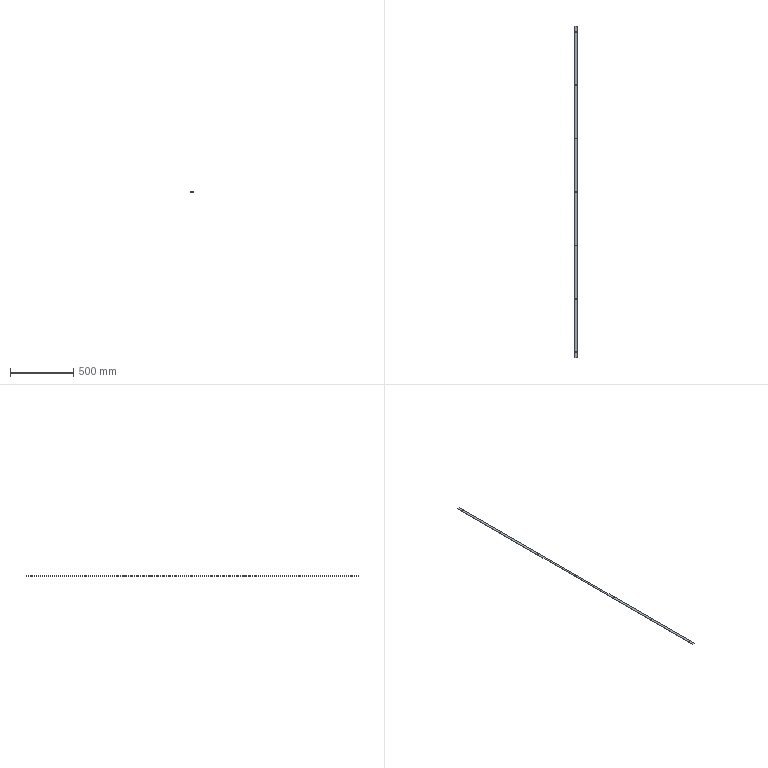Part | 1 solid | 20 faces | box 20 x 2616 x 1.5 mm | volume 78163 mm3 | cylinder 14 | plane 6 | commonest cylinder face diameters 6.2 x14
STEP:
#1=CARTESIAN_POINT('',(-3.1,-1263.,-1.5));
#2=VERTEX_POINT('',#1);
#3=CARTESIAN_POINT('',(3.1,-1263.,-1.5));
#4=VERTEX_POINT('',#3);
#5=CARTESIAN_POINT('',(0.,-1263.,-1.5));
#6=DIRECTION('',(0.,0.,1.));
#7=DIRECTION('',(1.,0.,0.));
#8=AXIS2_PLACEMENT_3D('',#5,#6,#7);
#9=CIRCLE('',#8,3.1);
#10=EDGE_CURVE('',#2,#4,#9,.T.);
#11=ORIENTED_EDGE('',*,*,#10,.F.);
#12=CARTESIAN_POINT('',(-3.1,-1263.,0.));
#13=VERTEX_POINT('',#12);
#14=CARTESIAN_POINT('',(-3.1,-1263.,-10.));
#15=DIRECTION('',(0.,0.,1.));
#16=VECTOR('',#15,1000.);
#17=LINE('',#14,#16);
#18=EDGE_CURVE('',#2,#13,#17,.T.);
#19=ORIENTED_EDGE('',*,*,#18,.T.);
#20=CARTESIAN_POINT('',(3.1,-1263.,0.));
#21=VERTEX_POINT('',#20);
#22=CARTESIAN_POINT('',(0.,-1263.,0.));
#23=DIRECTION('',(0.,0.,1.));
#24=DIRECTION('',(-1.,0.,0.));
#25=AXIS2_PLACEMENT_3D('',#22,#23,#24);
#26=CIRCLE('',#25,3.1);
#27=EDGE_CURVE('',#13,#21,#26,.T.);
#28=ORIENTED_EDGE('',*,*,#27,.T.);
#29=CARTESIAN_POINT('',(3.1,-1263.,-10.));
#30=DIRECTION('',(0.,0.,1.));
#31=VECTOR('',#30,1000.);
#32=LINE('',#29,#31);
#33=EDGE_CURVE('',#4,#21,#32,.T.);
#34=ORIENTED_EDGE('',*,*,#33,.F.);
#35=EDGE_LOOP('',(#11,#19,#28,#34));
#36=FACE_OUTER_BOUND('',#35,.T.);
#37=CARTESIAN_POINT('',(0.,-1263.,-10.));
#38=DIRECTION('',(0.,0.,1.));
#39=DIRECTION('',(1.,0.,0.));
#40=AXIS2_PLACEMENT_3D('',#37,#38,#39);
#41=CYLINDRICAL_SURFACE('',#40,3.1);
#42=ADVANCED_FACE('',(#36),#41,.F.);
#43=CARTESIAN_POINT('',(-3.1,-842.,-1.5));
#44=VERTEX_POINT('',#43);
#45=CARTESIAN_POINT('',(3.1,-842.,-1.5));
#46=VERTEX_POINT('',#45);
#47=CARTESIAN_POINT('',(0.,-842.,-1.5));
#48=DIRECTION('',(0.,0.,1.));
#49=DIRECTION('',(1.,0.,0.));
#50=AXIS2_PLACEMENT_3D('',#47,#48,#49);
#51=CIRCLE('',#50,3.1);
#52=EDGE_CURVE('',#44,#46,#51,.T.);
#53=ORIENTED_EDGE('',*,*,#52,.F.);
#54=CARTESIAN_POINT('',(-3.1,-842.,0.));
#55=VERTEX_POINT('',#54);
#56=CARTESIAN_POINT('',(-3.1,-842.,-10.));
#57=DIRECTION('',(0.,0.,1.));
#58=VECTOR('',#57,1000.);
#59=LINE('',#56,#58);
#60=EDGE_CURVE('',#44,#55,#59,.T.);
#61=ORIENTED_EDGE('',*,*,#60,.T.);
#62=CARTESIAN_POINT('',(3.1,-842.,0.));
#63=VERTEX_POINT('',#62);
#64=CARTESIAN_POINT('',(0.,-842.,0.));
#65=DIRECTION('',(0.,0.,1.));
#66=DIRECTION('',(-1.,0.,0.));
#67=AXIS2_PLACEMENT_3D('',#64,#65,#66);
#68=CIRCLE('',#67,3.1);
#69=EDGE_CURVE('',#55,#63,#68,.T.);
#70=ORIENTED_EDGE('',*,*,#69,.T.);
#71=CARTESIAN_POINT('',(3.1,-842.,-10.));
#72=DIRECTION('',(0.,0.,1.));
#73=VECTOR('',#72,1000.);
#74=LINE('',#71,#73);
#75=EDGE_CURVE('',#46,#63,#74,.T.);
#76=ORIENTED_EDGE('',*,*,#75,.F.);
#77=EDGE_LOOP('',(#53,#61,#70,#76));
#78=FACE_OUTER_BOUND('',#77,.T.);
#79=CARTESIAN_POINT('',(0.,-842.,-10.));
#80=DIRECTION('',(0.,0.,1.));
#81=DIRECTION('',(1.,0.,0.));
#82=AXIS2_PLACEMENT_3D('',#79,#80,#81);
#83=CYLINDRICAL_SURFACE('',#82,3.1);
#84=ADVANCED_FACE('',(#78),#83,.F.);
#85=CARTESIAN_POINT('',(-3.1,421.,-1.5));
#86=VERTEX_POINT('',#85);
#87=CARTESIAN_POINT('',(3.1,421.,-1.5));
#88=VERTEX_POINT('',#87);
#89=CARTESIAN_POINT('',(0.,421.,-1.5));
#90=DIRECTION('',(0.,0.,1.));
#91=DIRECTION('',(1.,0.,0.));
#92=AXIS2_PLACEMENT_3D('',#89,#90,#91);
#93=CIRCLE('',#92,3.1);
#94=EDGE_CURVE('',#86,#88,#93,.T.);
#95=ORIENTED_EDGE('',*,*,#94,.F.);
#96=CARTESIAN_POINT('',(-3.1,421.,0.));
#97=VERTEX_POINT('',#96);
#98=CARTESIAN_POINT('',(-3.1,421.,-10.));
#99=DIRECTION('',(0.,0.,1.));
#100=VECTOR('',#99,1000.);
#101=LINE('',#98,#100);
#102=EDGE_CURVE('',#86,#97,#101,.T.);
#103=ORIENTED_EDGE('',*,*,#102,.T.);
#104=CARTESIAN_POINT('',(3.1,421.,0.));
#105=VERTEX_POINT('',#104);
#106=CARTESIAN_POINT('',(0.,421.,0.));
#107=DIRECTION('',(0.,0.,1.));
#108=DIRECTION('',(1.,0.,0.));
#109=AXIS2_PLACEMENT_3D('',#106,#107,#108);
#110=CIRCLE('',#109,3.1);
#111=EDGE_CURVE('',#97,#105,#110,.T.);
#112=ORIENTED_EDGE('',*,*,#111,.T.);
#113=CARTESIAN_POINT('',(3.1,421.,-10.));
#114=DIRECTION('',(0.,0.,1.));
#115=VECTOR('',#114,1000.);
#116=LINE('',#113,#115);
#117=EDGE_CURVE('',#88,#105,#116,.T.);
#118=ORIENTED_EDGE('',*,*,#117,.F.);
#119=EDGE_LOOP('',(#95,#103,#112,#118));
#120=FACE_OUTER_BOUND('',#119,.T.);
#121=CARTESIAN_POINT('',(0.,421.,-10.));
#122=DIRECTION('',(0.,0.,1.));
#123=DIRECTION('',(1.,0.,0.));
#124=AXIS2_PLACEMENT_3D('',#121,#122,#123);
#125=CYLINDRICAL_SURFACE('',#124,3.1);
#126=ADVANCED_FACE('',(#120),#125,.F.);
#127=CARTESIAN_POINT('',(-3.1,842.,-1.5));
#128=VERTEX_POINT('',#127);
#129=CARTESIAN_POINT('',(3.1,842.,-1.5));
#130=VERTEX_POINT('',#129);
#131=CARTESIAN_POINT('',(0.,842.,-1.5));
#132=DIRECTION('',(0.,0.,1.));
#133=DIRECTION('',(1.,0.,0.));
#134=AXIS2_PLACEMENT_3D('',#131,#132,#133);
#135=CIRCLE('',#134,3.1);
#136=EDGE_CURVE('',#128,#130,#135,.T.);
#137=ORIENTED_EDGE('',*,*,#136,.F.);
#138=CARTESIAN_POINT('',(-3.1,842.,0.));
#139=VERTEX_POINT('',#138);
#140=CARTESIAN_POINT('',(-3.1,842.,-10.));
#141=DIRECTION('',(0.,0.,1.));
#142=VECTOR('',#141,1000.);
#143=LINE('',#140,#142);
#144=EDGE_CURVE('',#128,#139,#143,.T.);
#145=ORIENTED_EDGE('',*,*,#144,.T.);
#146=CARTESIAN_POINT('',(3.1,842.,0.));
#147=VERTEX_POINT('',#146);
#148=CARTESIAN_POINT('',(0.,842.,0.));
#149=DIRECTION('',(0.,0.,1.));
#150=DIRECTION('',(1.,0.,0.));
#151=AXIS2_PLACEMENT_3D('',#148,#149,#150);
#152=CIRCLE('',#151,3.1);
#153=EDGE_CURVE('',#139,#147,#152,.T.);
#154=ORIENTED_EDGE('',*,*,#153,.T.);
#155=CARTESIAN_POINT('',(3.1,842.,-10.));
#156=DIRECTION('',(0.,0.,1.));
#157=VECTOR('',#156,1000.);
#158=LINE('',#155,#157);
#159=EDGE_CURVE('',#130,#147,#158,.T.);
#160=ORIENTED_EDGE('',*,*,#159,.F.);
#161=EDGE_LOOP('',(#137,#145,#154,#160));
#162=FACE_OUTER_BOUND('',#161,.T.);
#163=CARTESIAN_POINT('',(0.,842.,-10.));
#164=DIRECTION('',(0.,0.,1.));
#165=DIRECTION('',(1.,0.,0.));
#166=AXIS2_PLACEMENT_3D('',#163,#164,#165);
#167=CYLINDRICAL_SURFACE('',#166,3.1);
#168=ADVANCED_FACE('',(#162),#167,.F.);
#169=CARTESIAN_POINT('',(-3.1,1263.,-1.5));
#170=VERTEX_POINT('',#169);
#171=CARTESIAN_POINT('',(3.1,1263.,-1.5));
#172=VERTEX_POINT('',#171);
#173=CARTESIAN_POINT('',(0.,1263.,-1.5));
#174=DIRECTION('',(0.,0.,1.));
#175=DIRECTION('',(1.,0.,0.));
#176=AXIS2_PLACEMENT_3D('',#173,#174,#175);
#177=CIRCLE('',#176,3.1);
#178=EDGE_CURVE('',#170,#172,#177,.T.);
#179=ORIENTED_EDGE('',*,*,#178,.F.);
#180=CARTESIAN_POINT('',(-3.1,1263.,0.));
#181=VERTEX_POINT('',#180);
#182=CARTESIAN_POINT('',(-3.1,1263.,-10.));
#183=DIRECTION('',(0.,0.,1.));
#184=VECTOR('',#183,1000.);
#185=LINE('',#182,#184);
#186=EDGE_CURVE('',#170,#181,#185,.T.);
#187=ORIENTED_EDGE('',*,*,#186,.T.);
#188=CARTESIAN_POINT('',(3.1,1263.,0.));
#189=VERTEX_POINT('',#188);
#190=CARTESIAN_POINT('',(0.,1263.,0.));
#191=DIRECTION('',(0.,0.,1.));
#192=DIRECTION('',(1.,0.,0.));
#193=AXIS2_PLACEMENT_3D('',#190,#191,#192);
#194=CIRCLE('',#193,3.1);
#195=EDGE_CURVE('',#181,#189,#194,.T.);
#196=ORIENTED_EDGE('',*,*,#195,.T.);
#197=CARTESIAN_POINT('',(3.1,1263.,-10.));
#198=DIRECTION('',(0.,0.,1.));
#199=VECTOR('',#198,1000.);
#200=LINE('',#197,#199);
#201=EDGE_CURVE('',#172,#189,#200,.T.);
#202=ORIENTED_EDGE('',*,*,#201,.F.);
#203=EDGE_LOOP('',(#179,#187,#196,#202));
#204=FACE_OUTER_BOUND('',#203,.T.);
#205=CARTESIAN_POINT('',(0.,1263.,-10.));
#206=DIRECTION('',(0.,0.,1.));
#207=DIRECTION('',(1.,0.,0.));
#208=AXIS2_PLACEMENT_3D('',#205,#206,#207);
#209=CYLINDRICAL_SURFACE('',#208,3.1);
#210=ADVANCED_FACE('',(#204),#209,.F.);
#211=CARTESIAN_POINT('',(-3.1,-421.,-1.5));
#212=VERTEX_POINT('',#211);
#213=CARTESIAN_POINT('',(3.1,-421.,-1.5));
#214=VERTEX_POINT('',#213);
#215=CARTESIAN_POINT('',(0.,-421.,-1.5));
#216=DIRECTION('',(0.,0.,1.));
#217=DIRECTION('',(1.,0.,0.));
#218=AXIS2_PLACEMENT_3D('',#215,#216,#217);
#219=CIRCLE('',#218,3.1);
#220=EDGE_CURVE('',#212,#214,#219,.T.);
#221=ORIENTED_EDGE('',*,*,#220,.F.);
#222=CARTESIAN_POINT('',(-3.1,-421.,0.));
#223=VERTEX_POINT('',#222);
#224=CARTESIAN_POINT('',(-3.1,-421.,-10.));
#225=DIRECTION('',(0.,0.,1.));
#226=VECTOR('',#225,1000.);
#227=LINE('',#224,#226);
#228=EDGE_CURVE('',#212,#223,#227,.T.);
#229=ORIENTED_EDGE('',*,*,#228,.T.);
#230=CARTESIAN_POINT('',(3.1,-421.,0.));
#231=VERTEX_POINT('',#230);
#232=CARTESIAN_POINT('',(0.,-421.,0.));
#233=DIRECTION('',(0.,0.,1.));
#234=DIRECTION('',(-1.,0.,0.));
#235=AXIS2_PLACEMENT_3D('',#232,#233,#234);
#236=CIRCLE('',#235,3.1);
#237=EDGE_CURVE('',#223,#231,#236,.T.);
#238=ORIENTED_EDGE('',*,*,#237,.T.);
#239=CARTESIAN_POINT('',(3.1,-421.,-10.));
#240=DIRECTION('',(0.,0.,1.));
#241=VECTOR('',#240,1000.);
#242=LINE('',#239,#241);
#243=EDGE_CURVE('',#214,#231,#242,.T.);
#244=ORIENTED_EDGE('',*,*,#243,.F.);
#245=EDGE_LOOP('',(#221,#229,#238,#244));
#246=FACE_OUTER_BOUND('',#245,.T.);
#247=CARTESIAN_POINT('',(0.,-421.,-10.));
#248=DIRECTION('',(0.,0.,1.));
#249=DIRECTION('',(1.,0.,0.));
#250=AXIS2_PLACEMENT_3D('',#247,#248,#249);
#251=CYLINDRICAL_SURFACE('',#250,3.1);
#252=ADVANCED_FACE('',(#246),#251,.F.);
#253=CARTESIAN_POINT('',(-3.1,0.,-1.5));
#254=VERTEX_POINT('',#253);
#255=CARTESIAN_POINT('',(3.1,0.,-1.5));
#256=VERTEX_POINT('',#255);
#257=CARTESIAN_POINT('',(0.,0.,-1.5));
#258=DIRECTION('',(0.,0.,1.));
#259=DIRECTION('',(1.,0.,0.));
#260=AXIS2_PLACEMENT_3D('',#257,#258,#259);
#261=CIRCLE('',#260,3.1);
#262=EDGE_CURVE('',#254,#256,#261,.T.);
#263=ORIENTED_EDGE('',*,*,#262,.F.);
#264=CARTESIAN_POINT('',(-3.1,0.,0.));
#265=VERTEX_POINT('',#264);
#266=CARTESIAN_POINT('',(-3.1,0.,-10.));
#267=DIRECTION('',(0.,0.,1.));
#268=VECTOR('',#267,1000.);
#269=LINE('',#266,#268);
#270=EDGE_CURVE('',#254,#265,#269,.T.);
#271=ORIENTED_EDGE('',*,*,#270,.T.);
#272=CARTESIAN_POINT('',(3.1,0.,0.));
#273=VERTEX_POINT('',#272);
#274=CARTESIAN_POINT('',(0.,0.,0.));
#275=DIRECTION('',(0.,0.,1.));
#276=DIRECTION('',(1.,0.,0.));
#277=AXIS2_PLACEMENT_3D('',#274,#275,#276);
#278=CIRCLE('',#277,3.1);
#279=EDGE_CURVE('',#265,#273,#278,.T.);
#280=ORIENTED_EDGE('',*,*,#279,.T.);
#281=CARTESIAN_POINT('',(3.1,0.,-10.));
#282=DIRECTION('',(0.,0.,1.));
#283=VECTOR('',#282,1000.);
#284=LINE('',#281,#283);
#285=EDGE_CURVE('',#256,#273,#284,.T.);
#286=ORIENTED_EDGE('',*,*,#285,.F.);
#287=EDGE_LOOP('',(#263,#271,#280,#286));
#288=FACE_OUTER_BOUND('',#287,.T.);
#289=CARTESIAN_POINT('',(0.,0.,-10.));
#290=DIRECTION('',(0.,0.,1.));
#291=DIRECTION('',(1.,0.,0.));
#292=AXIS2_PLACEMENT_3D('',#289,#290,#291);
#293=CYLINDRICAL_SURFACE('',#292,3.1);
#294=ADVANCED_FACE('',(#288),#293,.F.);
#295=CARTESIAN_POINT('',(10.,-1308.,0.));
#296=VERTEX_POINT('',#295);
#297=CARTESIAN_POINT('',(10.,1308.,0.));
#298=VERTEX_POINT('',#297);
#299=CARTESIAN_POINT('',(10.,1308.,0.));
#300=DIRECTION('',(0.,1.,0.));
#301=VECTOR('',#300,1000.);
#302=LINE('',#299,#301);
#303=EDGE_CURVE('',#296,#298,#302,.T.);
#304=ORIENTED_EDGE('',*,*,#303,.F.);
#305=CARTESIAN_POINT('',(10.,-1308.,-1.5));
#306=VERTEX_POINT('',#305);
#307=CARTESIAN_POINT('',(10.,-1308.,-1.5));
#308=DIRECTION('',(0.,0.,1.));
#309=VECTOR('',#308,1000.);
#310=LINE('',#307,#309);
#311=EDGE_CURVE('',#306,#296,#310,.T.);
#312=ORIENTED_EDGE('',*,*,#311,.F.);
#313=CARTESIAN_POINT('',(10.,1308.,-1.5));
#314=VERTEX_POINT('',#313);
#315=CARTESIAN_POINT('',(10.,1308.,-1.5));
#316=DIRECTION('',(0.,1.,0.));
#317=VECTOR('',#316,1000.);
#318=LINE('',#315,#317);
#319=EDGE_CURVE('',#306,#314,#318,.T.);
#320=ORIENTED_EDGE('',*,*,#319,.T.);
#321=CARTESIAN_POINT('',(10.,1308.,-1.5));
#322=DIRECTION('',(0.,0.,1.));
#323=VECTOR('',#322,1000.);
#324=LINE('',#321,#323);
#325=EDGE_CURVE('',#314,#298,#324,.T.);
#326=ORIENTED_EDGE('',*,*,#325,.T.);
#327=EDGE_LOOP('',(#304,#312,#320,#326));
#328=FACE_OUTER_BOUND('',#327,.T.);
#329=CARTESIAN_POINT('',(10.,1308.,-1.5));
#330=DIRECTION('',(1.,0.,0.));
#331=DIRECTION('',(0.,1.,0.));
#332=AXIS2_PLACEMENT_3D('',#329,#330,#331);
#333=PLANE('',#332);
#334=ADVANCED_FACE('',(#328),#333,.T.);
#335=CARTESIAN_POINT('',(-10.,-1308.,0.));
#336=VERTEX_POINT('',#335);
#337=CARTESIAN_POINT('',(-10.,-1308.,0.));
#338=DIRECTION('',(1.,0.,0.));
#339=VECTOR('',#338,1000.);
#340=LINE('',#337,#339);
#341=EDGE_CURVE('',#336,#296,#340,.T.);
#342=ORIENTED_EDGE('',*,*,#341,.F.);
#343=CARTESIAN_POINT('',(-10.,-1308.,-1.5));
#344=VERTEX_POINT('',#343);
#345=CARTESIAN_POINT('',(-10.,-1308.,-1.5));
#346=DIRECTION('',(0.,0.,1.));
#347=VECTOR('',#346,1000.);
#348=LINE('',#345,#347);
#349=EDGE_CURVE('',#344,#336,#348,.T.);
#350=ORIENTED_EDGE('',*,*,#349,.F.);
#351=CARTESIAN_POINT('',(-10.,-1308.,-1.5));
#352=DIRECTION('',(1.,0.,0.));
#353=VECTOR('',#352,1000.);
#354=LINE('',#351,#353);
#355=EDGE_CURVE('',#344,#306,#354,.T.);
#356=ORIENTED_EDGE('',*,*,#355,.T.);
#357=ORIENTED_EDGE('',*,*,#311,.T.);
#358=EDGE_LOOP('',(#342,#350,#356,#357));
#359=FACE_OUTER_BOUND('',#358,.T.);
#360=CARTESIAN_POINT('',(-10.,-1308.,-1.5));
#361=DIRECTION('',(0.,-1.,0.));
#362=DIRECTION('',(0.,0.,-1.));
#363=AXIS2_PLACEMENT_3D('',#360,#361,#362);
#364=PLANE('',#363);
#365=ADVANCED_FACE('',(#359),#364,.T.);
#366=CARTESIAN_POINT('',(-10.,1308.,0.));
#367=VERTEX_POINT('',#366);
#368=CARTESIAN_POINT('',(-10.,1308.,0.));
#369=DIRECTION('',(0.,-1.,0.));
#370=VECTOR('',#369,1000.);
#371=LINE('',#368,#370);
#372=EDGE_CURVE('',#367,#336,#371,.T.);
#373=ORIENTED_EDGE('',*,*,#372,.F.);
#374=CARTESIAN_POINT('',(-10.,1308.,-1.5));
#375=VERTEX_POINT('',#374);
#376=CARTESIAN_POINT('',(-10.,1308.,-1.5));
#377=DIRECTION('',(0.,0.,1.));
#378=VECTOR('',#377,1000.);
#379=LINE('',#376,#378);
#380=EDGE_CURVE('',#375,#367,#379,.T.);
#381=ORIENTED_EDGE('',*,*,#380,.F.);
#382=CARTESIAN_POINT('',(-10.,1308.,-1.5));
#383=DIRECTION('',(0.,-1.,0.));
#384=VECTOR('',#383,1000.);
#385=LINE('',#382,#384);
#386=EDGE_CURVE('',#375,#344,#385,.T.);
#387=ORIENTED_EDGE('',*,*,#386,.T.);
#388=ORIENTED_EDGE('',*,*,#349,.T.);
#389=EDGE_LOOP('',(#373,#381,#387,#388));
#390=FACE_OUTER_BOUND('',#389,.T.);
#391=CARTESIAN_POINT('',(-10.,1308.,-1.5));
#392=DIRECTION('',(-1.,0.,0.));
#393=DIRECTION('',(0.,-1.,0.));
#394=AXIS2_PLACEMENT_3D('',#391,#392,#393);
#395=PLANE('',#394);
#396=ADVANCED_FACE('',(#390),#395,.T.);
#397=CARTESIAN_POINT('',(-10.,1308.,0.));
#398=DIRECTION('',(-1.,0.,0.));
#399=VECTOR('',#398,1000.);
#400=LINE('',#397,#399);
#401=EDGE_CURVE('',#298,#367,#400,.T.);
#402=ORIENTED_EDGE('',*,*,#401,.F.);
#403=ORIENTED_EDGE('',*,*,#325,.F.);
#404=CARTESIAN_POINT('',(-10.,1308.,-1.5));
#405=DIRECTION('',(-1.,0.,0.));
#406=VECTOR('',#405,1000.);
#407=LINE('',#404,#406);
#408=EDGE_CURVE('',#314,#375,#407,.T.);
#409=ORIENTED_EDGE('',*,*,#408,.T.);
#410=ORIENTED_EDGE('',*,*,#380,.T.);
#411=EDGE_LOOP('',(#402,#403,#409,#410));
#412=FACE_OUTER_BOUND('',#411,.T.);
#413=CARTESIAN_POINT('',(-10.,1308.,-1.5));
#414=DIRECTION('',(0.,1.,0.));
#415=DIRECTION('',(0.,0.,1.));
#416=AXIS2_PLACEMENT_3D('',#413,#414,#415);
#417=PLANE('',#416);
#418=ADVANCED_FACE('',(#412),#417,.T.);
#419=CARTESIAN_POINT('',(0.,-1263.,-1.5));
#420=DIRECTION('',(0.,0.,1.));
#421=DIRECTION('',(1.,0.,0.));
#422=AXIS2_PLACEMENT_3D('',#419,#420,#421);
#423=CIRCLE('',#422,3.1);
#424=EDGE_CURVE('',#4,#2,#423,.T.);
#425=ORIENTED_EDGE('',*,*,#424,.T.);
#426=ORIENTED_EDGE('',*,*,#10,.T.);
#427=EDGE_LOOP('',(#425,#426));
#428=FACE_BOUND('',#427,.T.);
#429=CARTESIAN_POINT('',(0.,-842.,-1.5));
#430=DIRECTION('',(0.,0.,1.));
#431=DIRECTION('',(1.,0.,0.));
#432=AXIS2_PLACEMENT_3D('',#429,#430,#431);
#433=CIRCLE('',#432,3.1);
#434=EDGE_CURVE('',#46,#44,#433,.T.);
#435=ORIENTED_EDGE('',*,*,#434,.T.);
#436=ORIENTED_EDGE('',*,*,#52,.T.);
#437=EDGE_LOOP('',(#435,#436));
#438=FACE_BOUND('',#437,.T.);
#439=CARTESIAN_POINT('',(0.,421.,-1.5));
#440=DIRECTION('',(0.,0.,1.));
#441=DIRECTION('',(1.,0.,0.));
#442=AXIS2_PLACEMENT_3D('',#439,#440,#441);
#443=CIRCLE('',#442,3.1);
#444=EDGE_CURVE('',#88,#86,#443,.T.);
#445=ORIENTED_EDGE('',*,*,#444,.T.);
#446=ORIENTED_EDGE('',*,*,#94,.T.);
#447=EDGE_LOOP('',(#445,#446));
#448=FACE_BOUND('',#447,.T.);
#449=CARTESIAN_POINT('',(0.,842.,-1.5));
#450=DIRECTION('',(0.,0.,1.));
#451=DIRECTION('',(1.,0.,0.));
#452=AXIS2_PLACEMENT_3D('',#449,#450,#451);
#453=CIRCLE('',#452,3.1);
#454=EDGE_CURVE('',#130,#128,#453,.T.);
#455=ORIENTED_EDGE('',*,*,#454,.T.);
#456=ORIENTED_EDGE('',*,*,#136,.T.);
#457=EDGE_LOOP('',(#455,#456));
#458=FACE_BOUND('',#457,.T.);
#459=CARTESIAN_POINT('',(0.,1263.,-1.5));
#460=DIRECTION('',(0.,0.,1.));
#461=DIRECTION('',(1.,0.,0.));
#462=AXIS2_PLACEMENT_3D('',#459,#460,#461);
#463=CIRCLE('',#462,3.1);
#464=EDGE_CURVE('',#172,#170,#463,.T.);
#465=ORIENTED_EDGE('',*,*,#464,.T.);
#466=ORIENTED_EDGE('',*,*,#178,.T.);
#467=EDGE_LOOP('',(#465,#466));
#468=FACE_BOUND('',#467,.T.);
#469=CARTESIAN_POINT('',(0.,-421.,-1.5));
#470=DIRECTION('',(0.,0.,1.));
#471=DIRECTION('',(1.,0.,0.));
#472=AXIS2_PLACEMENT_3D('',#469,#470,#471);
#473=CIRCLE('',#472,3.1);
#474=EDGE_CURVE('',#214,#212,#473,.T.);
#475=ORIENTED_EDGE('',*,*,#474,.T.);
#476=ORIENTED_EDGE('',*,*,#220,.T.);
#477=EDGE_LOOP('',(#475,#476));
#478=FACE_BOUND('',#477,.T.);
#479=CARTESIAN_POINT('',(0.,0.,-1.5));
#480=DIRECTION('',(0.,0.,1.));
#481=DIRECTION('',(1.,0.,0.));
#482=AXIS2_PLACEMENT_3D('',#479,#480,#481);
#483=CIRCLE('',#482,3.1);
#484=EDGE_CURVE('',#256,#254,#483,.T.);
#485=ORIENTED_EDGE('',*,*,#484,.T.);
#486=ORIENTED_EDGE('',*,*,#262,.T.);
#487=EDGE_LOOP('',(#485,#486));
#488=FACE_BOUND('',#487,.T.);
#489=ORIENTED_EDGE('',*,*,#319,.F.);
#490=ORIENTED_EDGE('',*,*,#355,.F.);
#491=ORIENTED_EDGE('',*,*,#386,.F.);
#492=ORIENTED_EDGE('',*,*,#408,.F.);
#493=EDGE_LOOP('',(#489,#490,#491,#492));
#494=FACE_OUTER_BOUND('',#493,.T.);
#495=CARTESIAN_POINT('',(0.,0.,-1.5));
#496=DIRECTION('',(0.,0.,1.));
#497=DIRECTION('',(1.,0.,0.));
#498=AXIS2_PLACEMENT_3D('',#495,#496,#497);
#499=PLANE('',#498);
#500=ADVANCED_FACE('',(#428,#438,#448,#458,#468,#478,#488,#494),#499,.F.);
#501=CARTESIAN_POINT('',(0.,-1263.,0.));
#502=DIRECTION('',(0.,0.,1.));
#503=DIRECTION('',(-1.,0.,0.));
#504=AXIS2_PLACEMENT_3D('',#501,#502,#503);
#505=CIRCLE('',#504,3.1);
#506=EDGE_CURVE('',#21,#13,#505,.T.);
#507=ORIENTED_EDGE('',*,*,#506,.F.);
#508=ORIENTED_EDGE('',*,*,#27,.F.);
#509=EDGE_LOOP('',(#507,#508));
#510=FACE_BOUND('',#509,.T.);
#511=CARTESIAN_POINT('',(0.,-842.,0.));
#512=DIRECTION('',(0.,0.,1.));
#513=DIRECTION('',(-1.,0.,0.));
#514=AXIS2_PLACEMENT_3D('',#511,#512,#513);
#515=CIRCLE('',#514,3.1);
#516=EDGE_CURVE('',#63,#55,#515,.T.);
#517=ORIENTED_EDGE('',*,*,#516,.F.);
#518=ORIENTED_EDGE('',*,*,#69,.F.);
#519=EDGE_LOOP('',(#517,#518));
#520=FACE_BOUND('',#519,.T.);
#521=CARTESIAN_POINT('',(0.,421.,0.));
#522=DIRECTION('',(0.,0.,1.));
#523=DIRECTION('',(1.,0.,0.));
#524=AXIS2_PLACEMENT_3D('',#521,#522,#523);
#525=CIRCLE('',#524,3.1);
#526=EDGE_CURVE('',#105,#97,#525,.T.);
#527=ORIENTED_EDGE('',*,*,#526,.F.);
#528=ORIENTED_EDGE('',*,*,#111,.F.);
#529=EDGE_LOOP('',(#527,#528));
#530=FACE_BOUND('',#529,.T.);
#531=CARTESIAN_POINT('',(0.,842.,0.));
#532=DIRECTION('',(0.,0.,1.));
#533=DIRECTION('',(1.,0.,0.));
#534=AXIS2_PLACEMENT_3D('',#531,#532,#533);
#535=CIRCLE('',#534,3.1);
#536=EDGE_CURVE('',#147,#139,#535,.T.);
#537=ORIENTED_EDGE('',*,*,#536,.F.);
#538=ORIENTED_EDGE('',*,*,#153,.F.);
#539=EDGE_LOOP('',(#537,#538));
#540=FACE_BOUND('',#539,.T.);
#541=CARTESIAN_POINT('',(0.,1263.,0.));
#542=DIRECTION('',(0.,0.,1.));
#543=DIRECTION('',(1.,0.,0.));
#544=AXIS2_PLACEMENT_3D('',#541,#542,#543);
#545=CIRCLE('',#544,3.1);
#546=EDGE_CURVE('',#189,#181,#545,.T.);
#547=ORIENTED_EDGE('',*,*,#546,.F.);
#548=ORIENTED_EDGE('',*,*,#195,.F.);
#549=EDGE_LOOP('',(#547,#548));
#550=FACE_BOUND('',#549,.T.);
#551=CARTESIAN_POINT('',(0.,-421.,0.));
#552=DIRECTION('',(0.,0.,1.));
#553=DIRECTION('',(-1.,0.,0.));
#554=AXIS2_PLACEMENT_3D('',#551,#552,#553);
#555=CIRCLE('',#554,3.1);
#556=EDGE_CURVE('',#231,#223,#555,.T.);
#557=ORIENTED_EDGE('',*,*,#556,.F.);
#558=ORIENTED_EDGE('',*,*,#237,.F.);
#559=EDGE_LOOP('',(#557,#558));
#560=FACE_BOUND('',#559,.T.);
#561=CARTESIAN_POINT('',(0.,0.,0.));
#562=DIRECTION('',(0.,0.,1.));
#563=DIRECTION('',(1.,0.,0.));
#564=AXIS2_PLACEMENT_3D('',#561,#562,#563);
#565=CIRCLE('',#564,3.1);
#566=EDGE_CURVE('',#273,#265,#565,.T.);
#567=ORIENTED_EDGE('',*,*,#566,.F.);
#568=ORIENTED_EDGE('',*,*,#279,.F.);
#569=EDGE_LOOP('',(#567,#568));
#570=FACE_BOUND('',#569,.T.);
#571=ORIENTED_EDGE('',*,*,#303,.T.);
#572=ORIENTED_EDGE('',*,*,#401,.T.);
#573=ORIENTED_EDGE('',*,*,#372,.T.);
#574=ORIENTED_EDGE('',*,*,#341,.T.);
#575=EDGE_LOOP('',(#571,#572,#573,#574));
#576=FACE_OUTER_BOUND('',#575,.T.);
#577=CARTESIAN_POINT('',(0.,0.,0.));
#578=DIRECTION('',(0.,0.,1.));
#579=DIRECTION('',(1.,0.,0.));
#580=AXIS2_PLACEMENT_3D('',#577,#578,#579);
#581=PLANE('',#580);
#582=ADVANCED_FACE('',(#510,#520,#530,#540,#550,#560,#570,#576),#581,.T.);
#583=ORIENTED_EDGE('',*,*,#270,.F.);
#584=ORIENTED_EDGE('',*,*,#484,.F.);
#585=ORIENTED_EDGE('',*,*,#285,.T.);
#586=ORIENTED_EDGE('',*,*,#566,.T.);
#587=EDGE_LOOP('',(#583,#584,#585,#586));
#588=FACE_OUTER_BOUND('',#587,.T.);
#589=CARTESIAN_POINT('',(0.,0.,-10.));
#590=DIRECTION('',(0.,0.,1.));
#591=DIRECTION('',(1.,0.,0.));
#592=AXIS2_PLACEMENT_3D('',#589,#590,#591);
#593=CYLINDRICAL_SURFACE('',#592,3.1);
#594=ADVANCED_FACE('',(#588),#593,.F.);
#595=ORIENTED_EDGE('',*,*,#228,.F.);
#596=ORIENTED_EDGE('',*,*,#474,.F.);
#597=ORIENTED_EDGE('',*,*,#243,.T.);
#598=ORIENTED_EDGE('',*,*,#556,.T.);
#599=EDGE_LOOP('',(#595,#596,#597,#598));
#600=FACE_OUTER_BOUND('',#599,.T.);
#601=CARTESIAN_POINT('',(0.,-421.,-10.));
#602=DIRECTION('',(0.,0.,1.));
#603=DIRECTION('',(1.,0.,0.));
#604=AXIS2_PLACEMENT_3D('',#601,#602,#603);
#605=CYLINDRICAL_SURFACE('',#604,3.1);
#606=ADVANCED_FACE('',(#600),#605,.F.);
#607=ORIENTED_EDGE('',*,*,#186,.F.);
#608=ORIENTED_EDGE('',*,*,#464,.F.);
#609=ORIENTED_EDGE('',*,*,#201,.T.);
#610=ORIENTED_EDGE('',*,*,#546,.T.);
#611=EDGE_LOOP('',(#607,#608,#609,#610));
#612=FACE_OUTER_BOUND('',#611,.T.);
#613=CARTESIAN_POINT('',(0.,1263.,-10.));
#614=DIRECTION('',(0.,0.,1.));
#615=DIRECTION('',(1.,0.,0.));
#616=AXIS2_PLACEMENT_3D('',#613,#614,#615);
#617=CYLINDRICAL_SURFACE('',#616,3.1);
#618=ADVANCED_FACE('',(#612),#617,.F.);
#619=ORIENTED_EDGE('',*,*,#144,.F.);
#620=ORIENTED_EDGE('',*,*,#454,.F.);
#621=ORIENTED_EDGE('',*,*,#159,.T.);
#622=ORIENTED_EDGE('',*,*,#536,.T.);
#623=EDGE_LOOP('',(#619,#620,#621,#622));
#624=FACE_OUTER_BOUND('',#623,.T.);
#625=CARTESIAN_POINT('',(0.,842.,-10.));
#626=DIRECTION('',(0.,0.,1.));
#627=DIRECTION('',(1.,0.,0.));
#628=AXIS2_PLACEMENT_3D('',#625,#626,#627);
#629=CYLINDRICAL_SURFACE('',#628,3.1);
#630=ADVANCED_FACE('',(#624),#629,.F.);
#631=ORIENTED_EDGE('',*,*,#102,.F.);
#632=ORIENTED_EDGE('',*,*,#444,.F.);
#633=ORIENTED_EDGE('',*,*,#117,.T.);
#634=ORIENTED_EDGE('',*,*,#526,.T.);
#635=EDGE_LOOP('',(#631,#632,#633,#634));
#636=FACE_OUTER_BOUND('',#635,.T.);
#637=CARTESIAN_POINT('',(0.,421.,-10.));
#638=DIRECTION('',(0.,0.,1.));
#639=DIRECTION('',(1.,0.,0.));
#640=AXIS2_PLACEMENT_3D('',#637,#638,#639);
#641=CYLINDRICAL_SURFACE('',#640,3.1);
#642=ADVANCED_FACE('',(#636),#641,.F.);
#643=ORIENTED_EDGE('',*,*,#60,.F.);
#644=ORIENTED_EDGE('',*,*,#434,.F.);
#645=ORIENTED_EDGE('',*,*,#75,.T.);
#646=ORIENTED_EDGE('',*,*,#516,.T.);
#647=EDGE_LOOP('',(#643,#644,#645,#646));
#648=FACE_OUTER_BOUND('',#647,.T.);
#649=CARTESIAN_POINT('',(0.,-842.,-10.));
#650=DIRECTION('',(0.,0.,1.));
#651=DIRECTION('',(1.,0.,0.));
#652=AXIS2_PLACEMENT_3D('',#649,#650,#651);
#653=CYLINDRICAL_SURFACE('',#652,3.1);
#654=ADVANCED_FACE('',(#648),#653,.F.);
#655=ORIENTED_EDGE('',*,*,#18,.F.);
#656=ORIENTED_EDGE('',*,*,#424,.F.);
#657=ORIENTED_EDGE('',*,*,#33,.T.);
#658=ORIENTED_EDGE('',*,*,#506,.T.);
#659=EDGE_LOOP('',(#655,#656,#657,#658));
#660=FACE_OUTER_BOUND('',#659,.T.);
#661=CARTESIAN_POINT('',(0.,-1263.,-10.));
#662=DIRECTION('',(0.,0.,1.));
#663=DIRECTION('',(1.,0.,0.));
#664=AXIS2_PLACEMENT_3D('',#661,#662,#663);
#665=CYLINDRICAL_SURFACE('',#664,3.1);
#666=ADVANCED_FACE('',(#660),#665,.F.);
#667=CLOSED_SHELL('',(#42,#84,#126,#168,#210,#252,#294,#334,#365,#396,#418,#500,#582,#594,#606,#618,#630,#642,#654,#666));
#668=MANIFOLD_SOLID_BREP('',#667);
#669=CARTESIAN_POINT('',(0.,0.,0.));
#670=DIRECTION('',(0.,0.,1.));
#671=DIRECTION('',(1.,0.,0.));
#672=AXIS2_PLACEMENT_3D('',#669,#670,#671);
#673=(LENGTH_UNIT()NAMED_UNIT(*)SI_UNIT(.MILLI.,.METRE.));
#674=UNCERTAINTY_MEASURE_WITH_UNIT(LENGTH_MEASURE(0.00001),#673,'','');
#675=(NAMED_UNIT(*)PLANE_ANGLE_UNIT()SI_UNIT($,.RADIAN.));
#676=(NAMED_UNIT(*)SI_UNIT($,.STERADIAN.)SOLID_ANGLE_UNIT());
#677=(GEOMETRIC_REPRESENTATION_CONTEXT(3)GLOBAL_UNCERTAINTY_ASSIGNED_CONTEXT((#674))GLOBAL_UNIT_ASSIGNED_CONTEXT((#673,#675,#676))REPRESENTATION_CONTEXT('',''));
#678=ADVANCED_BREP_SHAPE_REPRESENTATION('',(#668,#672),#677);